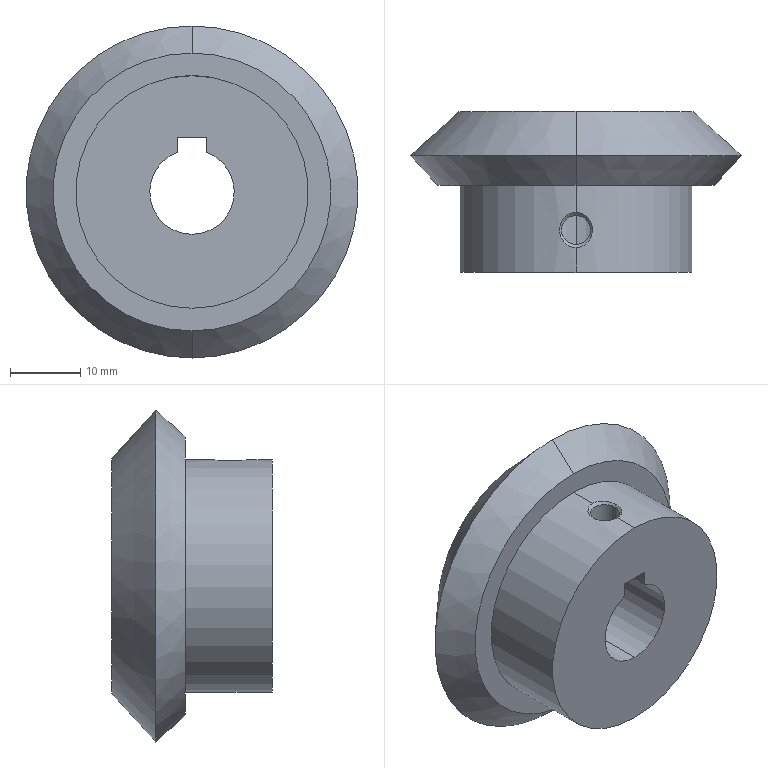Part | SolidWorks | features 3DProfileFeature 1, BaseBody 1 | 1 solid | 23 faces | box 47.12 x 22.819 x 47.12 mm | volume 20583 mm3 | plane 9 | cone 8 | cylinder 6 | commonest cylinder face diameters 4.134 x2 12 x2 33 x2
STEP:
#1=CARTESIAN_POINT('',(2.067,6.,5.633));
#2=VERTEX_POINT('',#1);
#3=CARTESIAN_POINT('',(2.,6.522,5.657));
#4=VERTEX_POINT('',#3);
#5=CARTESIAN_POINT('',(2.067,6.,5.633));
#6=CARTESIAN_POINT('',(2.067,6.175,5.633));
#7=CARTESIAN_POINT('',(2.044,6.352,5.641));
#8=CARTESIAN_POINT('',(2.,6.522,5.657));
#9=B_SPLINE_CURVE_WITH_KNOTS('',3,(#5,#6,#7,#8),.UNSPECIFIED.,.F.,.F.,(4,4),(0.0005265,0.001049),.UNSPECIFIED.);
#10=EDGE_CURVE('',#2,#4,#9,.T.);
#11=ORIENTED_EDGE('',*,*,#10,.F.);
#12=CARTESIAN_POINT('',(2.067,6.,16.067));
#13=VERTEX_POINT('',#12);
#14=CARTESIAN_POINT('',(2.067,6.,0.));
#15=DIRECTION('',(0.,0.,1.));
#16=VECTOR('',#15,1000.);
#17=LINE('',#14,#16);
#18=EDGE_CURVE('',#2,#13,#17,.T.);
#19=ORIENTED_EDGE('',*,*,#18,.T.);
#20=CARTESIAN_POINT('',(-2.067,6.,16.067));
#21=VERTEX_POINT('',#20);
#22=CARTESIAN_POINT('',(0.,6.,16.067));
#23=DIRECTION('',(0.,0.,-1.));
#24=DIRECTION('',(-1.,0.,0.));
#25=AXIS2_PLACEMENT_3D('',#22,#23,#24);
#26=CIRCLE('',#25,2.067);
#27=EDGE_CURVE('',#21,#13,#26,.T.);
#28=ORIENTED_EDGE('',*,*,#27,.F.);
#29=CARTESIAN_POINT('',(-2.067,6.,5.633));
#30=VERTEX_POINT('',#29);
#31=CARTESIAN_POINT('',(-2.067,6.,0.));
#32=DIRECTION('',(0.,0.,1.));
#33=VECTOR('',#32,1000.);
#34=LINE('',#31,#33);
#35=EDGE_CURVE('',#30,#21,#34,.T.);
#36=ORIENTED_EDGE('',*,*,#35,.F.);
#37=CARTESIAN_POINT('',(-2.,6.522,5.657));
#38=VERTEX_POINT('',#37);
#39=CARTESIAN_POINT('',(-2.,6.522,5.657));
#40=CARTESIAN_POINT('',(-2.045,6.35,5.641));
#41=CARTESIAN_POINT('',(-2.067,6.176,5.633));
#42=CARTESIAN_POINT('',(-2.067,6.,5.633));
#43=B_SPLINE_CURVE_WITH_KNOTS('',3,(#39,#40,#41,#42),.UNSPECIFIED.,.F.,.F.,(4,4),(0.,0.0005265),.UNSPECIFIED.);
#44=EDGE_CURVE('',#38,#30,#43,.T.);
#45=ORIENTED_EDGE('',*,*,#44,.F.);
#46=CARTESIAN_POINT('',(-2.,6.522,7.8));
#47=VERTEX_POINT('',#46);
#48=CARTESIAN_POINT('',(-2.,6.522,0.));
#49=DIRECTION('',(0.,0.,-1.));
#50=VECTOR('',#49,1000.);
#51=LINE('',#48,#50);
#52=EDGE_CURVE('',#47,#38,#51,.T.);
#53=ORIENTED_EDGE('',*,*,#52,.F.);
#54=CARTESIAN_POINT('',(2.,6.522,7.8));
#55=VERTEX_POINT('',#54);
#56=CARTESIAN_POINT('',(0.,6.,7.8));
#57=DIRECTION('',(0.,0.,1.));
#58=DIRECTION('',(-1.,0.,0.));
#59=AXIS2_PLACEMENT_3D('',#56,#57,#58);
#60=CIRCLE('',#59,2.067);
#61=EDGE_CURVE('',#55,#47,#60,.T.);
#62=ORIENTED_EDGE('',*,*,#61,.F.);
#63=CARTESIAN_POINT('',(2.,6.522,0.));
#64=DIRECTION('',(0.,0.,1.));
#65=VECTOR('',#64,1000.);
#66=LINE('',#63,#65);
#67=EDGE_CURVE('',#4,#55,#66,.T.);
#68=ORIENTED_EDGE('',*,*,#67,.F.);
#69=EDGE_LOOP('',(#11,#19,#28,#36,#45,#53,#62,#68));
#70=FACE_OUTER_BOUND('',#69,.T.);
#71=CARTESIAN_POINT('',(0.,6.,0.));
#72=DIRECTION('',(0.,0.,1.));
#73=DIRECTION('',(-1.,0.,0.));
#74=AXIS2_PLACEMENT_3D('',#71,#72,#73);
#75=CYLINDRICAL_SURFACE('',#74,2.067);
#76=ADVANCED_FACE('',(#70),#75,.F.);
#77=CARTESIAN_POINT('',(0.,6.,16.067));
#78=DIRECTION('',(0.,0.,-1.));
#79=DIRECTION('',(-1.,0.,0.));
#80=AXIS2_PLACEMENT_3D('',#77,#78,#79);
#81=CIRCLE('',#80,2.067);
#82=EDGE_CURVE('',#13,#21,#81,.T.);
#83=ORIENTED_EDGE('',*,*,#82,.T.);
#84=CARTESIAN_POINT('',(-2.334,6.,16.334));
#85=VERTEX_POINT('',#84);
#86=CARTESIAN_POINT('',(-2.5,6.,16.5));
#87=DIRECTION('',(-0.7071,0.,0.7071));
#88=VECTOR('',#87,1000.);
#89=LINE('',#86,#88);
#90=EDGE_CURVE('',#21,#85,#89,.T.);
#91=ORIENTED_EDGE('',*,*,#90,.T.);
#92=CARTESIAN_POINT('',(0.,3.5,16.5));
#93=VERTEX_POINT('',#92);
#94=CARTESIAN_POINT('',(-2.334,6.,16.334));
#95=CARTESIAN_POINT('',(-2.334,5.842,16.334));
#96=CARTESIAN_POINT('',(-2.32,5.682,16.336));
#97=CARTESIAN_POINT('',(-2.264,5.372,16.344));
#98=CARTESIAN_POINT('',(-2.222,5.22,16.35));
#99=CARTESIAN_POINT('',(-2.111,4.923,16.364));
#100=CARTESIAN_POINT('',(-2.042,4.779,16.373));
#101=CARTESIAN_POINT('',(-1.879,4.51,16.393));
#102=CARTESIAN_POINT('',(-1.785,4.383,16.404));
#103=CARTESIAN_POINT('',(-1.572,4.147,16.425));
#104=CARTESIAN_POINT('',(-1.456,4.04,16.436));
#105=CARTESIAN_POINT('',(-1.203,3.852,16.457));
#106=CARTESIAN_POINT('',(-1.065,3.77,16.466));
#107=CARTESIAN_POINT('',(-0.6354,3.572,16.49));
#108=CARTESIAN_POINT('',(-0.3194,3.5,16.5));
#109=CARTESIAN_POINT('',(0.,3.5,16.5));
#110=B_SPLINE_CURVE_WITH_KNOTS('',3,(#94,#95,#96,#97,#98,#99,#100,#101,#102,#103,#104,#105,#106,#107,#108,#109),.UNSPECIFIED.,.F.,.F.,(4,2,2,2,2,2,2,4),(0.0119,0.01238,0.01286,0.01334,0.01381,0.01429,0.01477,0.01572),.UNSPECIFIED.);
#111=EDGE_CURVE('',#85,#93,#110,.T.);
#112=ORIENTED_EDGE('',*,*,#111,.T.);
#113=CARTESIAN_POINT('',(2.334,6.,16.334));
#114=VERTEX_POINT('',#113);
#115=CARTESIAN_POINT('',(0.,3.5,16.5));
#116=CARTESIAN_POINT('',(0.16,3.5,16.5));
#117=CARTESIAN_POINT('',(0.3178,3.518,16.498));
#118=CARTESIAN_POINT('',(0.6256,3.586,16.489));
#119=CARTESIAN_POINT('',(0.778,3.637,16.482));
#120=CARTESIAN_POINT('',(1.066,3.77,16.466));
#121=CARTESIAN_POINT('',(1.201,3.851,16.457));
#122=CARTESIAN_POINT('',(1.454,4.039,16.436));
#123=CARTESIAN_POINT('',(1.573,4.147,16.425));
#124=CARTESIAN_POINT('',(1.784,4.381,16.404));
#125=CARTESIAN_POINT('',(1.877,4.508,16.393));
#126=CARTESIAN_POINT('',(2.041,4.778,16.373));
#127=CARTESIAN_POINT('',(2.111,4.923,16.365));
#128=CARTESIAN_POINT('',(2.222,5.218,16.35));
#129=CARTESIAN_POINT('',(2.263,5.37,16.344));
#130=CARTESIAN_POINT('',(2.32,5.683,16.336));
#131=CARTESIAN_POINT('',(2.334,5.842,16.334));
#132=CARTESIAN_POINT('',(2.334,6.,16.334));
#133=B_SPLINE_CURVE_WITH_KNOTS('',3,(#115,#116,#117,#118,#119,#120,#121,#122,#123,#124,#125,#126,#127,#128,#129,#130,#131,#132),.UNSPECIFIED.,.F.,.F.,(4,2,2,2,2,2,2,2,4),(0.0004392,0.000917,0.001395,0.001873,0.00235,0.002828,0.003306,0.003784,0.004261),.UNSPECIFIED.);
#134=EDGE_CURVE('',#93,#114,#133,.T.);
#135=ORIENTED_EDGE('',*,*,#134,.T.);
#136=CARTESIAN_POINT('',(2.5,6.,16.5));
#137=DIRECTION('',(0.7071,0.,0.7071));
#138=VECTOR('',#137,1000.);
#139=LINE('',#136,#138);
#140=EDGE_CURVE('',#13,#114,#139,.T.);
#141=ORIENTED_EDGE('',*,*,#140,.F.);
#142=EDGE_LOOP('',(#83,#91,#112,#135,#141));
#143=FACE_OUTER_BOUND('',#142,.T.);
#144=CARTESIAN_POINT('',(0.,6.,16.5));
#145=DIRECTION('',(0.,0.,1.));
#146=DIRECTION('',(1.,0.,0.));
#147=AXIS2_PLACEMENT_3D('',#144,#145,#146);
#148=CONICAL_SURFACE('',#147,2.5,0.7854);
#149=ADVANCED_FACE('',(#143),#148,.F.);
#150=CARTESIAN_POINT('',(0.,0.,16.5));
#151=VERTEX_POINT('',#150);
#152=CARTESIAN_POINT('',(0.,0.,-16.5));
#153=VERTEX_POINT('',#152);
#154=CARTESIAN_POINT('',(0.,0.,0.));
#155=DIRECTION('',(0.,-1.,0.));
#156=DIRECTION('',(0.,0.,-1.));
#157=AXIS2_PLACEMENT_3D('',#154,#155,#156);
#158=CIRCLE('',#157,16.5);
#159=EDGE_CURVE('',#151,#153,#158,.T.);
#160=ORIENTED_EDGE('',*,*,#159,.F.);
#161=CARTESIAN_POINT('',(0.,0.,16.5));
#162=DIRECTION('',(0.,1.,0.));
#163=VECTOR('',#162,1000.);
#164=LINE('',#161,#163);
#165=EDGE_CURVE('',#151,#93,#164,.T.);
#166=ORIENTED_EDGE('',*,*,#165,.T.);
#167=ORIENTED_EDGE('',*,*,#111,.F.);
#168=CARTESIAN_POINT('',(0.,8.5,16.5));
#169=VERTEX_POINT('',#168);
#170=CARTESIAN_POINT('',(0.,8.5,16.5));
#171=CARTESIAN_POINT('',(-0.1583,8.5,16.5));
#172=CARTESIAN_POINT('',(-0.3152,8.483,16.498));
#173=CARTESIAN_POINT('',(-0.6264,8.414,16.489));
#174=CARTESIAN_POINT('',(-0.7777,8.363,16.482));
#175=CARTESIAN_POINT('',(-1.064,8.231,16.466));
#176=CARTESIAN_POINT('',(-1.2,8.149,16.457));
#177=CARTESIAN_POINT('',(-1.456,7.96,16.436));
#178=CARTESIAN_POINT('',(-1.572,7.853,16.425));
#179=CARTESIAN_POINT('',(-1.783,7.62,16.404));
#180=CARTESIAN_POINT('',(-1.878,7.491,16.393));
#181=CARTESIAN_POINT('',(-2.042,7.22,16.373));
#182=CARTESIAN_POINT('',(-2.111,7.078,16.365));
#183=CARTESIAN_POINT('',(-2.221,6.782,16.35));
#184=CARTESIAN_POINT('',(-2.264,6.627,16.344));
#185=CARTESIAN_POINT('',(-2.32,6.315,16.336));
#186=CARTESIAN_POINT('',(-2.334,6.158,16.334));
#187=CARTESIAN_POINT('',(-2.334,6.,16.334));
#188=B_SPLINE_CURVE_WITH_KNOTS('',3,(#170,#171,#172,#173,#174,#175,#176,#177,#178,#179,#180,#181,#182,#183,#184,#185,#186,#187),.UNSPECIFIED.,.F.,.F.,(4,2,2,2,2,2,2,2,4),(0.008079,0.008557,0.009035,0.009513,0.009992,0.01047,0.01095,0.01143,0.0119),.UNSPECIFIED.);
#189=EDGE_CURVE('',#169,#85,#188,.T.);
#190=ORIENTED_EDGE('',*,*,#189,.F.);
#191=CARTESIAN_POINT('',(0.,12.34,16.5));
#192=VERTEX_POINT('',#191);
#193=CARTESIAN_POINT('',(0.,0.,16.5));
#194=DIRECTION('',(0.,1.,0.));
#195=VECTOR('',#194,1000.);
#196=LINE('',#193,#195);
#197=EDGE_CURVE('',#169,#192,#196,.T.);
#198=ORIENTED_EDGE('',*,*,#197,.T.);
#199=CARTESIAN_POINT('',(0.,12.34,-16.5));
#200=VERTEX_POINT('',#199);
#201=CARTESIAN_POINT('',(0.,12.34,0.));
#202=DIRECTION('',(0.,-1.,0.));
#203=DIRECTION('',(0.,0.,-1.));
#204=AXIS2_PLACEMENT_3D('',#201,#202,#203);
#205=CIRCLE('',#204,16.5);
#206=EDGE_CURVE('',#192,#200,#205,.T.);
#207=ORIENTED_EDGE('',*,*,#206,.T.);
#208=CARTESIAN_POINT('',(0.,0.,-16.5));
#209=DIRECTION('',(0.,1.,0.));
#210=VECTOR('',#209,1000.);
#211=LINE('',#208,#210);
#212=EDGE_CURVE('',#153,#200,#211,.T.);
#213=ORIENTED_EDGE('',*,*,#212,.F.);
#214=EDGE_LOOP('',(#160,#166,#167,#190,#198,#207,#213));
#215=FACE_OUTER_BOUND('',#214,.T.);
#216=CARTESIAN_POINT('',(0.,0.,0.));
#217=DIRECTION('',(0.,1.,0.));
#218=DIRECTION('',(0.,0.,-1.));
#219=AXIS2_PLACEMENT_3D('',#216,#217,#218);
#220=CYLINDRICAL_SURFACE('',#219,16.5);
#221=ADVANCED_FACE('',(#215),#220,.T.);
#222=CARTESIAN_POINT('',(0.,12.34,-19.72));
#223=VERTEX_POINT('',#222);
#224=CARTESIAN_POINT('',(0.,12.34,19.72));
#225=VERTEX_POINT('',#224);
#226=CARTESIAN_POINT('',(0.,12.34,0.));
#227=DIRECTION('',(0.,-1.,0.));
#228=DIRECTION('',(0.,0.,-1.));
#229=AXIS2_PLACEMENT_3D('',#226,#227,#228);
#230=CIRCLE('',#229,19.72);
#231=EDGE_CURVE('',#223,#225,#230,.T.);
#232=ORIENTED_EDGE('',*,*,#231,.F.);
#233=CARTESIAN_POINT('',(0.,16.56,-23.56));
#234=VERTEX_POINT('',#233);
#235=CARTESIAN_POINT('',(0.,16.56,-23.56));
#236=DIRECTION('',(0.,0.7396,-0.673));
#237=VECTOR('',#236,1000.);
#238=LINE('',#235,#237);
#239=EDGE_CURVE('',#223,#234,#238,.T.);
#240=ORIENTED_EDGE('',*,*,#239,.T.);
#241=CARTESIAN_POINT('',(0.,16.56,23.56));
#242=VERTEX_POINT('',#241);
#243=CARTESIAN_POINT('',(0.,16.56,0.));
#244=DIRECTION('',(0.,-1.,0.));
#245=DIRECTION('',(0.,0.,-1.));
#246=AXIS2_PLACEMENT_3D('',#243,#244,#245);
#247=CIRCLE('',#246,23.56);
#248=EDGE_CURVE('',#234,#242,#247,.T.);
#249=ORIENTED_EDGE('',*,*,#248,.T.);
#250=CARTESIAN_POINT('',(0.,16.56,23.56));
#251=DIRECTION('',(0.,0.7396,0.673));
#252=VECTOR('',#251,1000.);
#253=LINE('',#250,#252);
#254=EDGE_CURVE('',#225,#242,#253,.T.);
#255=ORIENTED_EDGE('',*,*,#254,.F.);
#256=EDGE_LOOP('',(#232,#240,#249,#255));
#257=FACE_OUTER_BOUND('',#256,.T.);
#258=CARTESIAN_POINT('',(0.,16.56,0.));
#259=DIRECTION('',(0.,1.,0.));
#260=DIRECTION('',(0.,0.,1.));
#261=AXIS2_PLACEMENT_3D('',#258,#259,#260);
#262=CONICAL_SURFACE('',#261,23.56,0.7383);
#263=ADVANCED_FACE('',(#257),#262,.T.);
#264=CARTESIAN_POINT('',(0.,22.819,-16.681));
#265=VERTEX_POINT('',#264);
#266=CARTESIAN_POINT('',(0.,22.819,16.681));
#267=VERTEX_POINT('',#266);
#268=CARTESIAN_POINT('',(0.,22.819,0.));
#269=DIRECTION('',(0.,-1.,0.));
#270=DIRECTION('',(0.,0.,-1.));
#271=AXIS2_PLACEMENT_3D('',#268,#269,#270);
#272=CIRCLE('',#271,16.681);
#273=EDGE_CURVE('',#265,#267,#272,.T.);
#274=ORIENTED_EDGE('',*,*,#273,.T.);
#275=CARTESIAN_POINT('',(0.,22.819,16.681));
#276=DIRECTION('',(0.,-0.673,0.7396));
#277=VECTOR('',#276,1000.);
#278=LINE('',#275,#277);
#279=EDGE_CURVE('',#267,#242,#278,.T.);
#280=ORIENTED_EDGE('',*,*,#279,.T.);
#281=ORIENTED_EDGE('',*,*,#248,.F.);
#282=CARTESIAN_POINT('',(0.,22.819,-16.681));
#283=DIRECTION('',(0.,-0.673,-0.7396));
#284=VECTOR('',#283,1000.);
#285=LINE('',#282,#284);
#286=EDGE_CURVE('',#265,#234,#285,.T.);
#287=ORIENTED_EDGE('',*,*,#286,.F.);
#288=EDGE_LOOP('',(#274,#280,#281,#287));
#289=FACE_OUTER_BOUND('',#288,.T.);
#290=CARTESIAN_POINT('',(0.,22.819,0.));
#291=DIRECTION('',(0.,-1.,0.));
#292=DIRECTION('',(0.,0.,-1.));
#293=AXIS2_PLACEMENT_3D('',#290,#291,#292);
#294=CONICAL_SURFACE('',#293,16.681,0.8325);
#295=ADVANCED_FACE('',(#289),#294,.T.);
#296=CARTESIAN_POINT('',(0.,20.751,14.8));
#297=VERTEX_POINT('',#296);
#298=CARTESIAN_POINT('',(0.,20.751,-14.8));
#299=VERTEX_POINT('',#298);
#300=CARTESIAN_POINT('',(0.,20.751,0.));
#301=DIRECTION('',(0.,-1.,0.));
#302=DIRECTION('',(0.,0.,-1.));
#303=AXIS2_PLACEMENT_3D('',#300,#301,#302);
#304=CIRCLE('',#303,14.8);
#305=EDGE_CURVE('',#297,#299,#304,.T.);
#306=ORIENTED_EDGE('',*,*,#305,.T.);
#307=CARTESIAN_POINT('',(0.,20.751,-14.8));
#308=DIRECTION('',(0.,0.7396,-0.673));
#309=VECTOR('',#308,1000.);
#310=LINE('',#307,#309);
#311=EDGE_CURVE('',#299,#265,#310,.T.);
#312=ORIENTED_EDGE('',*,*,#311,.T.);
#313=CARTESIAN_POINT('',(0.,22.819,0.));
#314=DIRECTION('',(0.,-1.,0.));
#315=DIRECTION('',(0.,0.,-1.));
#316=AXIS2_PLACEMENT_3D('',#313,#314,#315);
#317=CIRCLE('',#316,16.681);
#318=EDGE_CURVE('',#267,#265,#317,.T.);
#319=ORIENTED_EDGE('',*,*,#318,.F.);
#320=CARTESIAN_POINT('',(0.,20.751,14.8));
#321=DIRECTION('',(0.,0.7396,0.673));
#322=VECTOR('',#321,1000.);
#323=LINE('',#320,#322);
#324=EDGE_CURVE('',#297,#267,#323,.T.);
#325=ORIENTED_EDGE('',*,*,#324,.F.);
#326=EDGE_LOOP('',(#306,#312,#319,#325));
#327=FACE_OUTER_BOUND('',#326,.T.);
#328=CARTESIAN_POINT('',(0.,20.751,0.));
#329=DIRECTION('',(0.,1.,0.));
#330=DIRECTION('',(0.,0.,1.));
#331=AXIS2_PLACEMENT_3D('',#328,#329,#330);
#332=CONICAL_SURFACE('',#331,14.8,0.7383);
#333=ADVANCED_FACE('',(#327),#332,.F.);
#334=CARTESIAN_POINT('',(-2.,0.,5.657));
#335=VERTEX_POINT('',#334);
#336=CARTESIAN_POINT('',(0.,0.,-6.));
#337=VERTEX_POINT('',#336);
#338=CARTESIAN_POINT('',(0.,0.,0.));
#339=DIRECTION('',(0.,-1.,0.));
#340=DIRECTION('',(0.,0.,1.));
#341=AXIS2_PLACEMENT_3D('',#338,#339,#340);
#342=CIRCLE('',#341,6.);
#343=EDGE_CURVE('',#335,#337,#342,.T.);
#344=ORIENTED_EDGE('',*,*,#343,.T.);
#345=CARTESIAN_POINT('',(0.,20.751,-6.));
#346=VERTEX_POINT('',#345);
#347=CARTESIAN_POINT('',(0.,22.83,-6.));
#348=DIRECTION('',(0.,1.,0.));
#349=VECTOR('',#348,1000.);
#350=LINE('',#347,#349);
#351=EDGE_CURVE('',#337,#346,#350,.T.);
#352=ORIENTED_EDGE('',*,*,#351,.T.);
#353=CARTESIAN_POINT('',(-2.,20.751,5.657));
#354=VERTEX_POINT('',#353);
#355=CARTESIAN_POINT('',(0.,20.751,0.));
#356=DIRECTION('',(0.,1.,0.));
#357=DIRECTION('',(0.,0.,-1.));
#358=AXIS2_PLACEMENT_3D('',#355,#356,#357);
#359=CIRCLE('',#358,6.);
#360=EDGE_CURVE('',#346,#354,#359,.T.);
#361=ORIENTED_EDGE('',*,*,#360,.T.);
#362=CARTESIAN_POINT('',(-2.,22.83,5.657));
#363=DIRECTION('',(0.,-1.,0.));
#364=VECTOR('',#363,1000.);
#365=LINE('',#362,#364);
#366=EDGE_CURVE('',#354,#38,#365,.T.);
#367=ORIENTED_EDGE('',*,*,#366,.T.);
#368=ORIENTED_EDGE('',*,*,#44,.T.);
#369=CARTESIAN_POINT('',(-2.,5.478,5.657));
#370=VERTEX_POINT('',#369);
#371=CARTESIAN_POINT('',(-2.067,6.,5.633));
#372=CARTESIAN_POINT('',(-2.067,5.825,5.633));
#373=CARTESIAN_POINT('',(-2.044,5.648,5.641));
#374=CARTESIAN_POINT('',(-2.,5.478,5.657));
#375=B_SPLINE_CURVE_WITH_KNOTS('',3,(#371,#372,#373,#374),.UNSPECIFIED.,.F.,.F.,(4,4),(0.0005265,0.001049),.UNSPECIFIED.);
#376=EDGE_CURVE('',#30,#370,#375,.T.);
#377=ORIENTED_EDGE('',*,*,#376,.T.);
#378=CARTESIAN_POINT('',(-2.,22.83,5.657));
#379=DIRECTION('',(0.,-1.,0.));
#380=VECTOR('',#379,1000.);
#381=LINE('',#378,#380);
#382=EDGE_CURVE('',#370,#335,#381,.T.);
#383=ORIENTED_EDGE('',*,*,#382,.T.);
#384=EDGE_LOOP('',(#344,#352,#361,#367,#368,#377,#383));
#385=FACE_OUTER_BOUND('',#384,.T.);
#386=CARTESIAN_POINT('',(0.,22.83,0.));
#387=DIRECTION('',(0.,1.,0.));
#388=DIRECTION('',(0.,0.,-1.));
#389=AXIS2_PLACEMENT_3D('',#386,#387,#388);
#390=CYLINDRICAL_SURFACE('',#389,6.);
#391=ADVANCED_FACE('',(#385),#390,.F.);
#392=CARTESIAN_POINT('',(2.,5.478,7.8));
#393=VERTEX_POINT('',#392);
#394=CARTESIAN_POINT('',(2.,0.,7.8));
#395=VERTEX_POINT('',#394);
#396=CARTESIAN_POINT('',(2.,22.83,7.8));
#397=DIRECTION('',(0.,-1.,0.));
#398=VECTOR('',#397,1000.);
#399=LINE('',#396,#398);
#400=EDGE_CURVE('',#393,#395,#399,.T.);
#401=ORIENTED_EDGE('',*,*,#400,.F.);
#402=CARTESIAN_POINT('',(2.,5.478,5.657));
#403=VERTEX_POINT('',#402);
#404=CARTESIAN_POINT('',(2.,5.478,0.));
#405=DIRECTION('',(0.,0.,-1.));
#406=VECTOR('',#405,1000.);
#407=LINE('',#404,#406);
#408=EDGE_CURVE('',#393,#403,#407,.T.);
#409=ORIENTED_EDGE('',*,*,#408,.T.);
#410=CARTESIAN_POINT('',(2.,0.,5.657));
#411=VERTEX_POINT('',#410);
#412=CARTESIAN_POINT('',(2.,22.83,5.657));
#413=DIRECTION('',(0.,-1.,0.));
#414=VECTOR('',#413,1000.);
#415=LINE('',#412,#414);
#416=EDGE_CURVE('',#403,#411,#415,.T.);
#417=ORIENTED_EDGE('',*,*,#416,.T.);
#418=CARTESIAN_POINT('',(2.,0.,7.8));
#419=DIRECTION('',(0.,0.,-1.));
#420=VECTOR('',#419,1000.);
#421=LINE('',#418,#420);
#422=EDGE_CURVE('',#395,#411,#421,.T.);
#423=ORIENTED_EDGE('',*,*,#422,.F.);
#424=EDGE_LOOP('',(#401,#409,#417,#423));
#425=FACE_OUTER_BOUND('',#424,.T.);
#426=CARTESIAN_POINT('',(2.,22.83,7.8));
#427=DIRECTION('',(-1.,0.,0.));
#428=DIRECTION('',(0.,0.,1.));
#429=AXIS2_PLACEMENT_3D('',#426,#427,#428);
#430=PLANE('',#429);
#431=ADVANCED_FACE('',(#425),#430,.T.);
#432=ORIENTED_EDGE('',*,*,#351,.F.);
#433=CARTESIAN_POINT('',(0.,0.,0.));
#434=DIRECTION('',(0.,-1.,0.));
#435=DIRECTION('',(0.,0.,1.));
#436=AXIS2_PLACEMENT_3D('',#433,#434,#435);
#437=CIRCLE('',#436,6.);
#438=EDGE_CURVE('',#337,#411,#437,.T.);
#439=ORIENTED_EDGE('',*,*,#438,.T.);
#440=ORIENTED_EDGE('',*,*,#416,.F.);
#441=CARTESIAN_POINT('',(2.,5.478,5.657));
#442=CARTESIAN_POINT('',(2.045,5.65,5.641));
#443=CARTESIAN_POINT('',(2.067,5.824,5.633));
#444=CARTESIAN_POINT('',(2.067,6.,5.633));
#445=B_SPLINE_CURVE_WITH_KNOTS('',3,(#441,#442,#443,#444),.UNSPECIFIED.,.F.,.F.,(4,4),(0.,0.0005265),.UNSPECIFIED.);
#446=EDGE_CURVE('',#403,#2,#445,.T.);
#447=ORIENTED_EDGE('',*,*,#446,.T.);
#448=ORIENTED_EDGE('',*,*,#10,.T.);
#449=CARTESIAN_POINT('',(2.,20.751,5.657));
#450=VERTEX_POINT('',#449);
#451=CARTESIAN_POINT('',(2.,22.83,5.657));
#452=DIRECTION('',(0.,-1.,0.));
#453=VECTOR('',#452,1000.);
#454=LINE('',#451,#453);
#455=EDGE_CURVE('',#450,#4,#454,.T.);
#456=ORIENTED_EDGE('',*,*,#455,.F.);
#457=CARTESIAN_POINT('',(0.,20.751,0.));
#458=DIRECTION('',(0.,1.,0.));
#459=DIRECTION('',(0.,0.,-1.));
#460=AXIS2_PLACEMENT_3D('',#457,#458,#459);
#461=CIRCLE('',#460,6.);
#462=EDGE_CURVE('',#450,#346,#461,.T.);
#463=ORIENTED_EDGE('',*,*,#462,.T.);
#464=EDGE_LOOP('',(#432,#439,#440,#447,#448,#456,#463));
#465=FACE_OUTER_BOUND('',#464,.T.);
#466=CARTESIAN_POINT('',(0.,22.83,0.));
#467=DIRECTION('',(0.,1.,0.));
#468=DIRECTION('',(0.,0.,-1.));
#469=AXIS2_PLACEMENT_3D('',#466,#467,#468);
#470=CYLINDRICAL_SURFACE('',#469,6.);
#471=ADVANCED_FACE('',(#465),#470,.F.);
#472=ORIENTED_EDGE('',*,*,#61,.T.);
#473=CARTESIAN_POINT('',(-2.,20.751,7.8));
#474=VERTEX_POINT('',#473);
#475=CARTESIAN_POINT('',(-2.,22.83,7.8));
#476=DIRECTION('',(0.,-1.,0.));
#477=VECTOR('',#476,1000.);
#478=LINE('',#475,#477);
#479=EDGE_CURVE('',#474,#47,#478,.T.);
#480=ORIENTED_EDGE('',*,*,#479,.F.);
#481=CARTESIAN_POINT('',(2.,20.751,7.8));
#482=VERTEX_POINT('',#481);
#483=CARTESIAN_POINT('',(0.,20.751,7.8));
#484=DIRECTION('',(1.,0.,0.));
#485=VECTOR('',#484,1000.);
#486=LINE('',#483,#485);
#487=EDGE_CURVE('',#474,#482,#486,.T.);
#488=ORIENTED_EDGE('',*,*,#487,.T.);
#489=CARTESIAN_POINT('',(2.,22.83,7.8));
#490=DIRECTION('',(0.,-1.,0.));
#491=VECTOR('',#490,1000.);
#492=LINE('',#489,#491);
#493=EDGE_CURVE('',#482,#55,#492,.T.);
#494=ORIENTED_EDGE('',*,*,#493,.T.);
#495=EDGE_LOOP('',(#472,#480,#488,#494));
#496=FACE_OUTER_BOUND('',#495,.T.);
#497=CARTESIAN_POINT('',(-2.,22.83,7.8));
#498=DIRECTION('',(0.,0.,-1.));
#499=DIRECTION('',(0.,-1.,0.));
#500=AXIS2_PLACEMENT_3D('',#497,#498,#499);
#501=PLANE('',#500);
#502=ADVANCED_FACE('',(#496),#501,.T.);
#503=ORIENTED_EDGE('',*,*,#382,.F.);
#504=CARTESIAN_POINT('',(-2.,5.478,7.8));
#505=VERTEX_POINT('',#504);
#506=CARTESIAN_POINT('',(-2.,5.478,0.));
#507=DIRECTION('',(0.,0.,1.));
#508=VECTOR('',#507,1000.);
#509=LINE('',#506,#508);
#510=EDGE_CURVE('',#370,#505,#509,.T.);
#511=ORIENTED_EDGE('',*,*,#510,.T.);
#512=CARTESIAN_POINT('',(-2.,0.,7.8));
#513=VERTEX_POINT('',#512);
#514=CARTESIAN_POINT('',(-2.,22.83,7.8));
#515=DIRECTION('',(0.,-1.,0.));
#516=VECTOR('',#515,1000.);
#517=LINE('',#514,#516);
#518=EDGE_CURVE('',#505,#513,#517,.T.);
#519=ORIENTED_EDGE('',*,*,#518,.T.);
#520=CARTESIAN_POINT('',(-2.,0.,5.657));
#521=DIRECTION('',(0.,0.,1.));
#522=VECTOR('',#521,1000.);
#523=LINE('',#520,#522);
#524=EDGE_CURVE('',#335,#513,#523,.T.);
#525=ORIENTED_EDGE('',*,*,#524,.F.);
#526=EDGE_LOOP('',(#503,#511,#519,#525));
#527=FACE_OUTER_BOUND('',#526,.T.);
#528=CARTESIAN_POINT('',(-2.,22.83,5.657));
#529=DIRECTION('',(1.,0.,0.));
#530=DIRECTION('',(0.,0.,1.));
#531=AXIS2_PLACEMENT_3D('',#528,#529,#530);
#532=PLANE('',#531);
#533=ADVANCED_FACE('',(#527),#532,.T.);
#534=ORIENTED_EDGE('',*,*,#518,.F.);
#535=CARTESIAN_POINT('',(0.,6.,7.8));
#536=DIRECTION('',(0.,0.,1.));
#537=DIRECTION('',(-1.,0.,0.));
#538=AXIS2_PLACEMENT_3D('',#535,#536,#537);
#539=CIRCLE('',#538,2.067);
#540=EDGE_CURVE('',#505,#393,#539,.T.);
#541=ORIENTED_EDGE('',*,*,#540,.T.);
#542=ORIENTED_EDGE('',*,*,#400,.T.);
#543=CARTESIAN_POINT('',(-2.,0.,7.8));
#544=DIRECTION('',(1.,0.,0.));
#545=VECTOR('',#544,1000.);
#546=LINE('',#543,#545);
#547=EDGE_CURVE('',#513,#395,#546,.T.);
#548=ORIENTED_EDGE('',*,*,#547,.F.);
#549=EDGE_LOOP('',(#534,#541,#542,#548));
#550=FACE_OUTER_BOUND('',#549,.T.);
#551=CARTESIAN_POINT('',(-2.,22.83,7.8));
#552=DIRECTION('',(0.,0.,-1.));
#553=DIRECTION('',(0.,-1.,0.));
#554=AXIS2_PLACEMENT_3D('',#551,#552,#553);
#555=PLANE('',#554);
#556=ADVANCED_FACE('',(#550),#555,.T.);
#557=ORIENTED_EDGE('',*,*,#479,.T.);
#558=ORIENTED_EDGE('',*,*,#52,.T.);
#559=ORIENTED_EDGE('',*,*,#366,.F.);
#560=CARTESIAN_POINT('',(-2.,20.751,0.));
#561=DIRECTION('',(0.,0.,1.));
#562=VECTOR('',#561,1000.);
#563=LINE('',#560,#562);
#564=EDGE_CURVE('',#354,#474,#563,.T.);
#565=ORIENTED_EDGE('',*,*,#564,.T.);
#566=EDGE_LOOP('',(#557,#558,#559,#565));
#567=FACE_OUTER_BOUND('',#566,.T.);
#568=CARTESIAN_POINT('',(-2.,22.83,5.657));
#569=DIRECTION('',(1.,0.,0.));
#570=DIRECTION('',(0.,0.,1.));
#571=AXIS2_PLACEMENT_3D('',#568,#569,#570);
#572=PLANE('',#571);
#573=ADVANCED_FACE('',(#567),#572,.T.);
#574=CARTESIAN_POINT('',(2.,20.751,0.));
#575=DIRECTION('',(0.,0.,-1.));
#576=VECTOR('',#575,1000.);
#577=LINE('',#574,#576);
#578=EDGE_CURVE('',#482,#450,#577,.T.);
#579=ORIENTED_EDGE('',*,*,#578,.F.);
#580=ORIENTED_EDGE('',*,*,#487,.F.);
#581=ORIENTED_EDGE('',*,*,#564,.F.);
#582=ORIENTED_EDGE('',*,*,#360,.F.);
#583=ORIENTED_EDGE('',*,*,#462,.F.);
#584=EDGE_LOOP('',(#579,#580,#581,#582,#583));
#585=FACE_BOUND('',#584,.T.);
#586=ORIENTED_EDGE('',*,*,#305,.F.);
#587=CARTESIAN_POINT('',(0.,20.751,0.));
#588=DIRECTION('',(0.,-1.,0.));
#589=DIRECTION('',(0.,0.,-1.));
#590=AXIS2_PLACEMENT_3D('',#587,#588,#589);
#591=CIRCLE('',#590,14.8);
#592=EDGE_CURVE('',#299,#297,#591,.T.);
#593=ORIENTED_EDGE('',*,*,#592,.F.);
#594=EDGE_LOOP('',(#586,#593));
#595=FACE_OUTER_BOUND('',#594,.T.);
#596=CARTESIAN_POINT('',(0.,20.751,0.));
#597=DIRECTION('',(0.,-1.,0.));
#598=DIRECTION('',(0.,0.,-1.));
#599=AXIS2_PLACEMENT_3D('',#596,#597,#598);
#600=PLANE('',#599);
#601=ADVANCED_FACE('',(#585,#595),#600,.F.);
#602=ORIENTED_EDGE('',*,*,#422,.T.);
#603=ORIENTED_EDGE('',*,*,#438,.F.);
#604=ORIENTED_EDGE('',*,*,#343,.F.);
#605=ORIENTED_EDGE('',*,*,#524,.T.);
#606=ORIENTED_EDGE('',*,*,#547,.T.);
#607=EDGE_LOOP('',(#602,#603,#604,#605,#606));
#608=FACE_BOUND('',#607,.T.);
#609=CARTESIAN_POINT('',(0.,0.,0.));
#610=DIRECTION('',(0.,-1.,0.));
#611=DIRECTION('',(0.,0.,-1.));
#612=AXIS2_PLACEMENT_3D('',#609,#610,#611);
#613=CIRCLE('',#612,16.5);
#614=EDGE_CURVE('',#153,#151,#613,.T.);
#615=ORIENTED_EDGE('',*,*,#614,.T.);
#616=ORIENTED_EDGE('',*,*,#159,.T.);
#617=EDGE_LOOP('',(#615,#616));
#618=FACE_OUTER_BOUND('',#617,.T.);
#619=CARTESIAN_POINT('',(16.5,0.,0.));
#620=DIRECTION('',(0.,1.,0.));
#621=DIRECTION('',(1.,0.,0.));
#622=AXIS2_PLACEMENT_3D('',#619,#620,#621);
#623=PLANE('',#622);
#624=ADVANCED_FACE('',(#608,#618),#623,.F.);
#625=ORIENTED_EDGE('',*,*,#311,.F.);
#626=ORIENTED_EDGE('',*,*,#592,.T.);
#627=ORIENTED_EDGE('',*,*,#324,.T.);
#628=ORIENTED_EDGE('',*,*,#273,.F.);
#629=EDGE_LOOP('',(#625,#626,#627,#628));
#630=FACE_OUTER_BOUND('',#629,.T.);
#631=CARTESIAN_POINT('',(0.,20.751,0.));
#632=DIRECTION('',(0.,1.,0.));
#633=DIRECTION('',(0.,0.,1.));
#634=AXIS2_PLACEMENT_3D('',#631,#632,#633);
#635=CONICAL_SURFACE('',#634,14.8,0.7383);
#636=ADVANCED_FACE('',(#630),#635,.F.);
#637=ORIENTED_EDGE('',*,*,#279,.F.);
#638=ORIENTED_EDGE('',*,*,#318,.T.);
#639=ORIENTED_EDGE('',*,*,#286,.T.);
#640=CARTESIAN_POINT('',(0.,16.56,0.));
#641=DIRECTION('',(0.,-1.,0.));
#642=DIRECTION('',(0.,0.,-1.));
#643=AXIS2_PLACEMENT_3D('',#640,#641,#642);
#644=CIRCLE('',#643,23.56);
#645=EDGE_CURVE('',#242,#234,#644,.T.);
#646=ORIENTED_EDGE('',*,*,#645,.F.);
#647=EDGE_LOOP('',(#637,#638,#639,#646));
#648=FACE_OUTER_BOUND('',#647,.T.);
#649=CARTESIAN_POINT('',(0.,22.819,0.));
#650=DIRECTION('',(0.,-1.,0.));
#651=DIRECTION('',(0.,0.,-1.));
#652=AXIS2_PLACEMENT_3D('',#649,#650,#651);
#653=CONICAL_SURFACE('',#652,16.681,0.8325);
#654=ADVANCED_FACE('',(#648),#653,.T.);
#655=ORIENTED_EDGE('',*,*,#239,.F.);
#656=CARTESIAN_POINT('',(0.,12.34,0.));
#657=DIRECTION('',(0.,-1.,0.));
#658=DIRECTION('',(0.,0.,-1.));
#659=AXIS2_PLACEMENT_3D('',#656,#657,#658);
#660=CIRCLE('',#659,19.72);
#661=EDGE_CURVE('',#225,#223,#660,.T.);
#662=ORIENTED_EDGE('',*,*,#661,.F.);
#663=ORIENTED_EDGE('',*,*,#254,.T.);
#664=ORIENTED_EDGE('',*,*,#645,.T.);
#665=EDGE_LOOP('',(#655,#662,#663,#664));
#666=FACE_OUTER_BOUND('',#665,.T.);
#667=CARTESIAN_POINT('',(0.,16.56,0.));
#668=DIRECTION('',(0.,1.,0.));
#669=DIRECTION('',(0.,0.,1.));
#670=AXIS2_PLACEMENT_3D('',#667,#668,#669);
#671=CONICAL_SURFACE('',#670,23.56,0.7383);
#672=ADVANCED_FACE('',(#666),#671,.T.);
#673=CARTESIAN_POINT('',(0.,12.34,0.));
#674=DIRECTION('',(0.,-1.,0.));
#675=DIRECTION('',(0.,0.,-1.));
#676=AXIS2_PLACEMENT_3D('',#673,#674,#675);
#677=CIRCLE('',#676,16.5);
#678=EDGE_CURVE('',#200,#192,#677,.T.);
#679=ORIENTED_EDGE('',*,*,#678,.F.);
#680=ORIENTED_EDGE('',*,*,#206,.F.);
#681=EDGE_LOOP('',(#679,#680));
#682=FACE_BOUND('',#681,.T.);
#683=ORIENTED_EDGE('',*,*,#661,.T.);
#684=ORIENTED_EDGE('',*,*,#231,.T.);
#685=EDGE_LOOP('',(#683,#684));
#686=FACE_OUTER_BOUND('',#685,.T.);
#687=CARTESIAN_POINT('',(19.72,12.34,0.));
#688=DIRECTION('',(0.,1.,0.));
#689=DIRECTION('',(1.,0.,0.));
#690=AXIS2_PLACEMENT_3D('',#687,#688,#689);
#691=PLANE('',#690);
#692=ADVANCED_FACE('',(#682,#686),#691,.F.);
#693=ORIENTED_EDGE('',*,*,#455,.T.);
#694=ORIENTED_EDGE('',*,*,#67,.T.);
#695=ORIENTED_EDGE('',*,*,#493,.F.);
#696=ORIENTED_EDGE('',*,*,#578,.T.);
#697=EDGE_LOOP('',(#693,#694,#695,#696));
#698=FACE_OUTER_BOUND('',#697,.T.);
#699=CARTESIAN_POINT('',(2.,22.83,7.8));
#700=DIRECTION('',(-1.,0.,0.));
#701=DIRECTION('',(0.,0.,1.));
#702=AXIS2_PLACEMENT_3D('',#699,#700,#701);
#703=PLANE('',#702);
#704=ADVANCED_FACE('',(#698),#703,.T.);
#705=ORIENTED_EDGE('',*,*,#165,.F.);
#706=ORIENTED_EDGE('',*,*,#614,.F.);
#707=ORIENTED_EDGE('',*,*,#212,.T.);
#708=ORIENTED_EDGE('',*,*,#678,.T.);
#709=ORIENTED_EDGE('',*,*,#197,.F.);
#710=CARTESIAN_POINT('',(2.334,6.,16.334));
#711=CARTESIAN_POINT('',(2.334,6.315,16.334));
#712=CARTESIAN_POINT('',(2.277,6.634,16.343));
#713=CARTESIAN_POINT('',(2.111,7.076,16.364));
#714=CARTESIAN_POINT('',(2.042,7.22,16.373));
#715=CARTESIAN_POINT('',(1.878,7.491,16.393));
#716=CARTESIAN_POINT('',(1.784,7.618,16.404));
#717=CARTESIAN_POINT('',(1.573,7.852,16.425));
#718=CARTESIAN_POINT('',(1.455,7.961,16.436));
#719=CARTESIAN_POINT('',(1.201,8.149,16.457));
#720=CARTESIAN_POINT('',(1.066,8.23,16.466));
#721=CARTESIAN_POINT('',(0.7762,8.363,16.482));
#722=CARTESIAN_POINT('',(0.6264,8.414,16.489));
#723=CARTESIAN_POINT('',(0.3183,8.482,16.498));
#724=CARTESIAN_POINT('',(0.1579,8.5,16.5));
#725=CARTESIAN_POINT('',(0.,8.5,16.5));
#726=B_SPLINE_CURVE_WITH_KNOTS('',3,(#710,#711,#712,#713,#714,#715,#716,#717,#718,#719,#720,#721,#722,#723,#724,#725),.UNSPECIFIED.,.F.,.F.,(4,2,2,2,2,2,2,4),(0.004261,0.005216,0.005693,0.00617,0.006647,0.007124,0.007601,0.008079),.UNSPECIFIED.);
#727=EDGE_CURVE('',#114,#169,#726,.T.);
#728=ORIENTED_EDGE('',*,*,#727,.F.);
#729=ORIENTED_EDGE('',*,*,#134,.F.);
#730=EDGE_LOOP('',(#705,#706,#707,#708,#709,#728,#729));
#731=FACE_OUTER_BOUND('',#730,.T.);
#732=CARTESIAN_POINT('',(0.,0.,0.));
#733=DIRECTION('',(0.,1.,0.));
#734=DIRECTION('',(0.,0.,-1.));
#735=AXIS2_PLACEMENT_3D('',#732,#733,#734);
#736=CYLINDRICAL_SURFACE('',#735,16.5);
#737=ADVANCED_FACE('',(#731),#736,.T.);
#738=ORIENTED_EDGE('',*,*,#90,.F.);
#739=ORIENTED_EDGE('',*,*,#27,.T.);
#740=ORIENTED_EDGE('',*,*,#140,.T.);
#741=ORIENTED_EDGE('',*,*,#727,.T.);
#742=ORIENTED_EDGE('',*,*,#189,.T.);
#743=EDGE_LOOP('',(#738,#739,#740,#741,#742));
#744=FACE_OUTER_BOUND('',#743,.T.);
#745=CARTESIAN_POINT('',(0.,6.,16.5));
#746=DIRECTION('',(0.,0.,1.));
#747=DIRECTION('',(1.,0.,0.));
#748=AXIS2_PLACEMENT_3D('',#745,#746,#747);
#749=CONICAL_SURFACE('',#748,2.5,0.7854);
#750=ADVANCED_FACE('',(#744),#749,.F.);
#751=ORIENTED_EDGE('',*,*,#18,.F.);
#752=ORIENTED_EDGE('',*,*,#446,.F.);
#753=ORIENTED_EDGE('',*,*,#408,.F.);
#754=ORIENTED_EDGE('',*,*,#540,.F.);
#755=ORIENTED_EDGE('',*,*,#510,.F.);
#756=ORIENTED_EDGE('',*,*,#376,.F.);
#757=ORIENTED_EDGE('',*,*,#35,.T.);
#758=ORIENTED_EDGE('',*,*,#82,.F.);
#759=EDGE_LOOP('',(#751,#752,#753,#754,#755,#756,#757,#758));
#760=FACE_OUTER_BOUND('',#759,.T.);
#761=CARTESIAN_POINT('',(0.,6.,0.));
#762=DIRECTION('',(0.,0.,1.));
#763=DIRECTION('',(-1.,0.,0.));
#764=AXIS2_PLACEMENT_3D('',#761,#762,#763);
#765=CYLINDRICAL_SURFACE('',#764,2.067);
#766=ADVANCED_FACE('',(#760),#765,.F.);
#767=CLOSED_SHELL('',(#76,#149,#221,#263,#295,#333,#391,#431,#471,#502,#533,#556,#573,#601,#624,#636,#654,#672,#692,#704,#737,#750,#766));
#768=MANIFOLD_SOLID_BREP('',#767);
#769=CARTESIAN_POINT('',(0.,0.,0.));
#770=DIRECTION('',(0.,0.,1.));
#771=DIRECTION('',(1.,0.,0.));
#772=AXIS2_PLACEMENT_3D('',#769,#770,#771);
#773=(LENGTH_UNIT()NAMED_UNIT(*)SI_UNIT(.MILLI.,.METRE.));
#774=UNCERTAINTY_MEASURE_WITH_UNIT(LENGTH_MEASURE(0.00001),#773,'','');
#775=(NAMED_UNIT(*)PLANE_ANGLE_UNIT()SI_UNIT($,.RADIAN.));
#776=(NAMED_UNIT(*)SI_UNIT($,.STERADIAN.)SOLID_ANGLE_UNIT());
#777=(GEOMETRIC_REPRESENTATION_CONTEXT(3)GLOBAL_UNCERTAINTY_ASSIGNED_CONTEXT((#774))GLOBAL_UNIT_ASSIGNED_CONTEXT((#773,#775,#776))REPRESENTATION_CONTEXT('',''));
#778=ADVANCED_BREP_SHAPE_REPRESENTATION('',(#768,#772),#777);